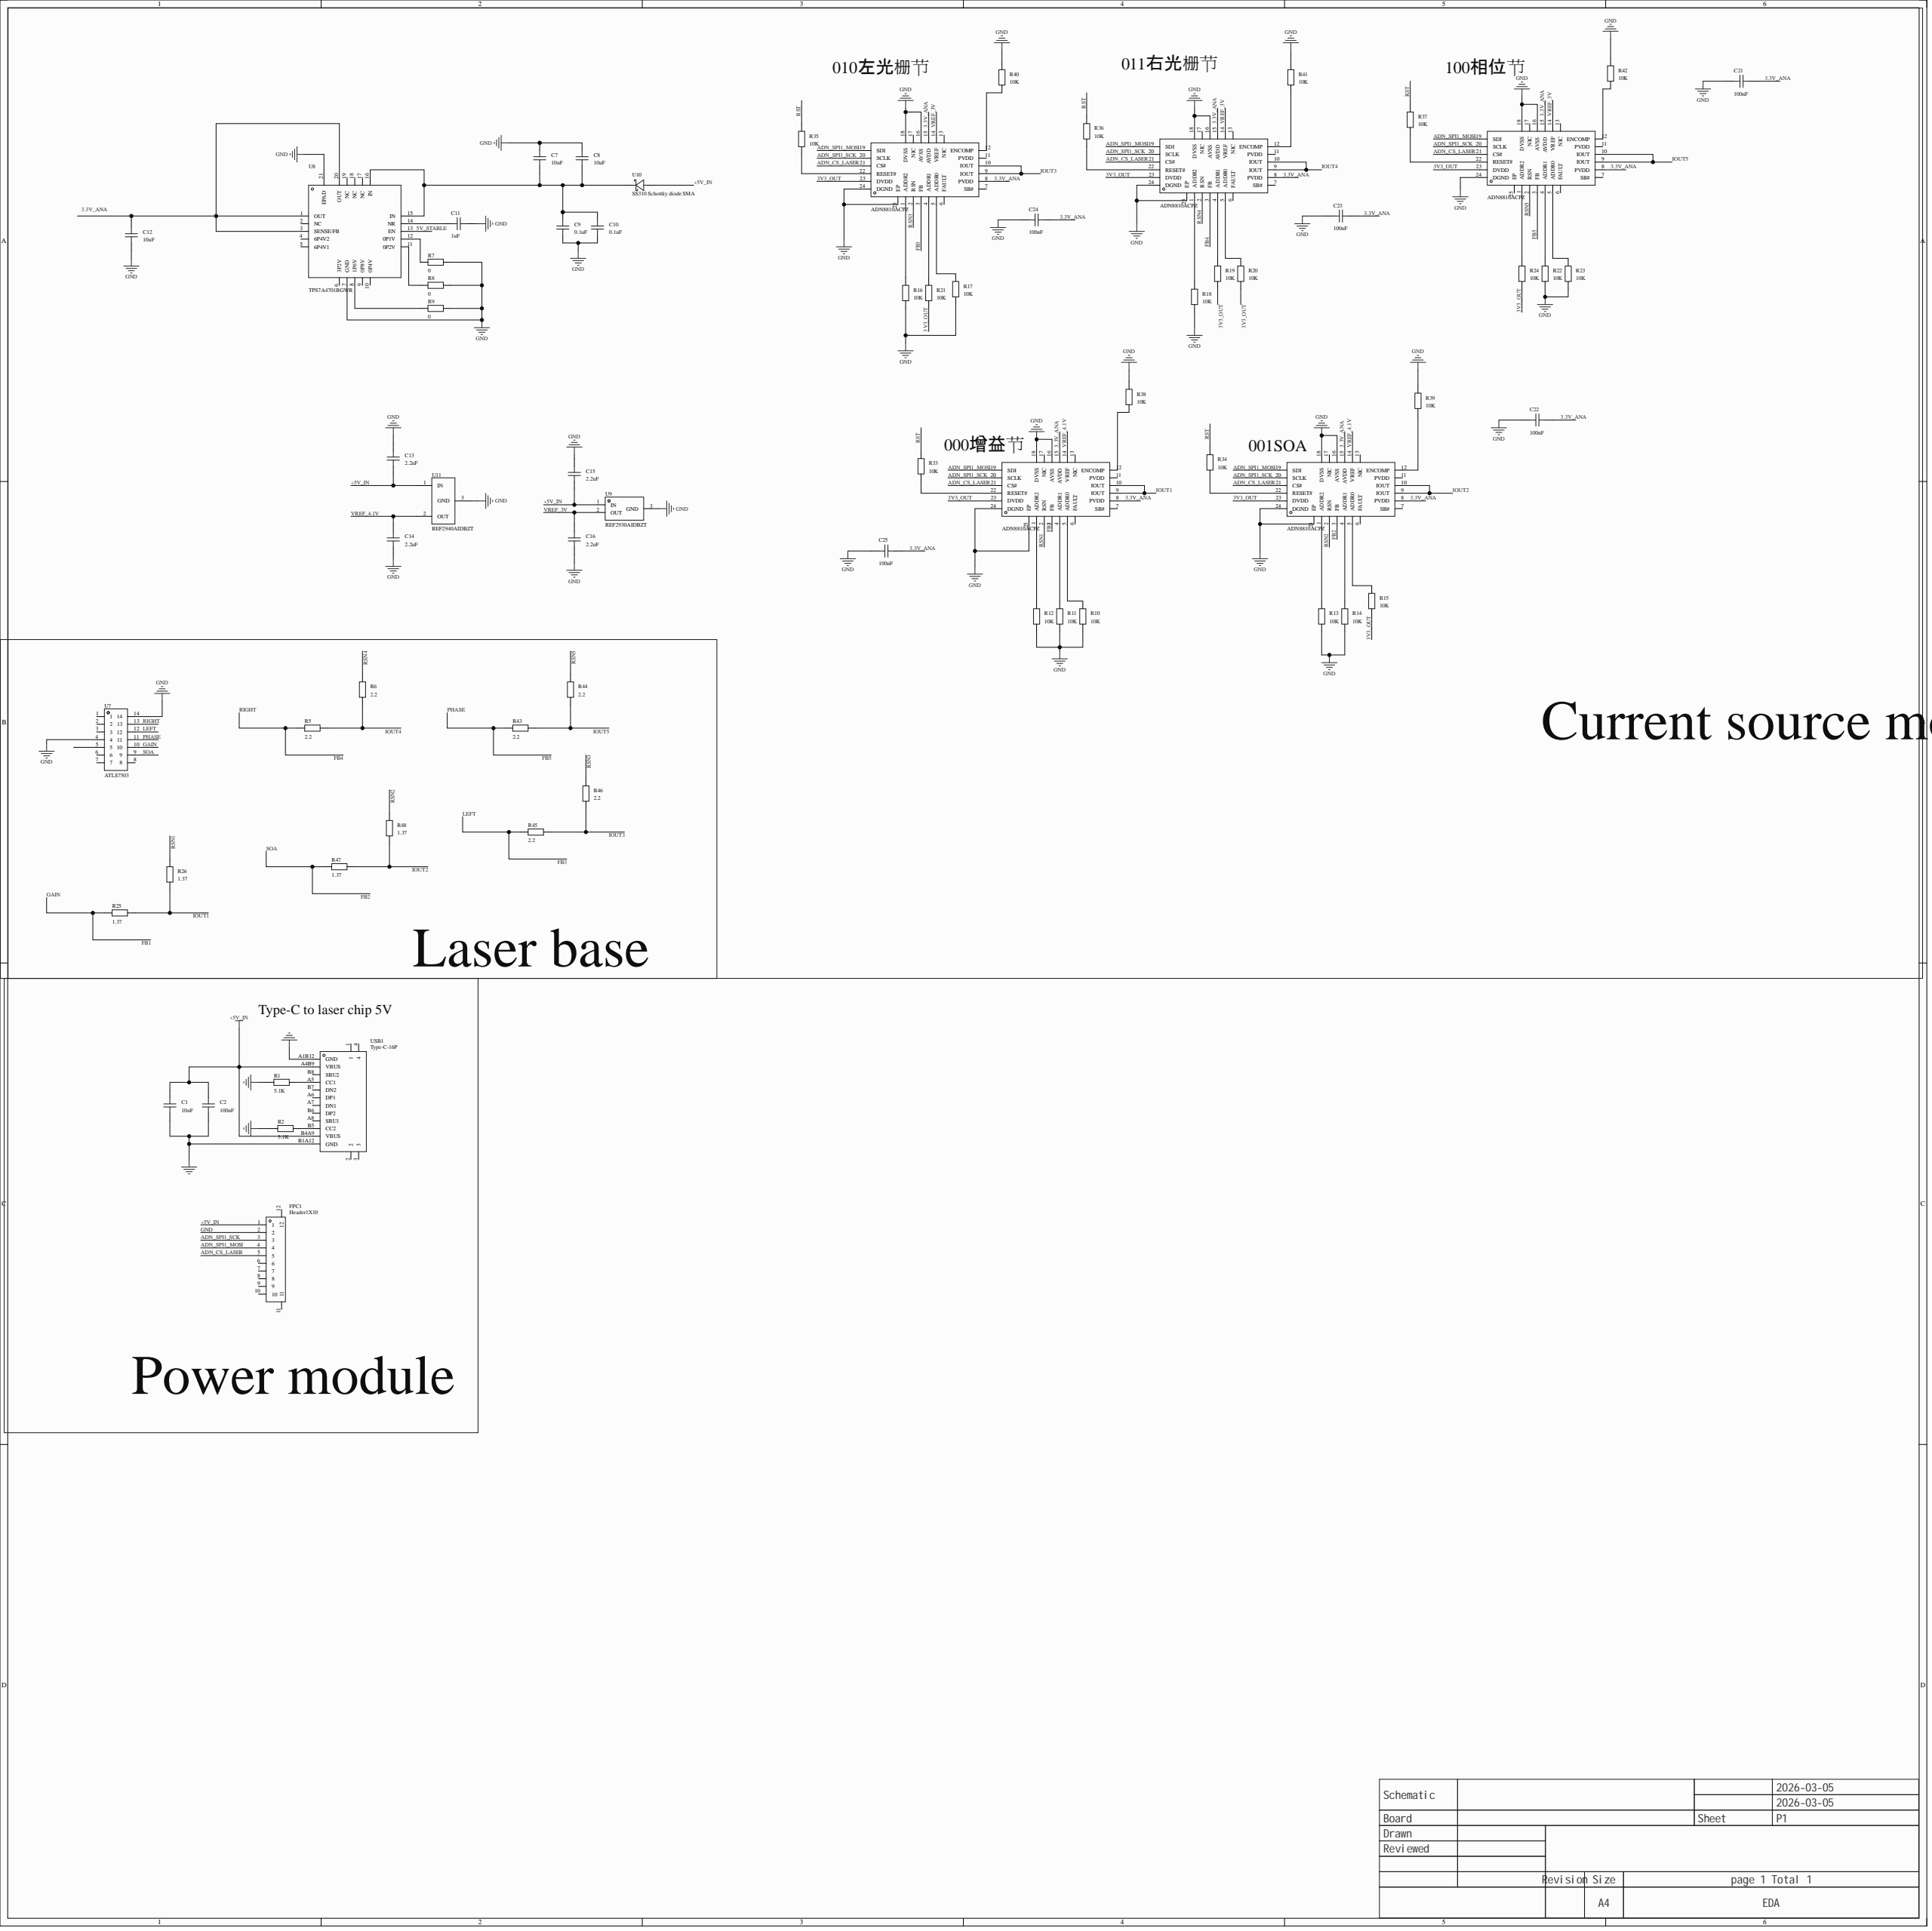Circuit board | Altium Designer | 69 parts | 58 nets
Bill of materials:
Comment,Description,Designator,Footprint,LibRef,Quantity
"ADN8810ACPZ","Output current: 300mA;","000增益节, 001SOA, 010左光栅节, 011右光栅节, 100相位节","LFCSP-24_L4.0-W4.0-P0.50-BL-EP2.3","ADN8810ACPZ","5"
"10uF","Capacitance: 10nF; accuracy: ±10%; rated voltage: 16V; temperature coefficient: X7R;","C1","C0402","AC0402KRX7R7BB103","1"
"100nF","Capacitance: 10nF; accuracy: ±10%; rated voltage: 16V; temperature coefficient: X7R;","C2","C0402","AC0402KRX7R7BB103","1"
"10uF","","C7, C8, C12","C0603","CAP_0603","3"
"0.1uF","","C9, C10","C0603","CAP_0603","2"
"1uF","","C11","C0603","CAP_0603","1"
"2.2uF","","C13, C14, C15, C16","C0603","CAP_0603","4"
"100nF","","C21, C22, C23, C24, C25","C0603","CAP_0603","5"
"Header1X10","","FPC1","FPC-SMD_10P-P1.00_C9900008955","Header1X10","1"
"5.1K","","R1, R2","R0603","Res_0603","2"
"2.2","","R5, R6, R43, R44, R45, R46","R0603","Res_0603","6"
"0","","R7, R8, R9","R0603","Res_0603","3"
"10K","","R10, R11, R12, R13, R14, R15, R16, R17, R18, R19, R20, R21, R22, R23, R24, R33, R34, R35, R36, R37, R38, R39, R40, R41, R42","R0603","Res_0603","25"
"1.37","","R25, R26, R47, R48","R0603","Res_0603","4"
"ATLS7503","","U7","HDR-SMD_14P-P1.27-V-F-R2-C7-LS4.8","HEADER7X2B","1"
"TPS7A4701RGWR","Output type: adjustable; working voltage: 35V; output voltage: 1.4V~34V; output current: 1A; power supply rejection ratio (PSRR): 78dB@(1kHz); output polarity: positive;","U8","VQFN-20_L5.0-W5.0-P0.65-TL-EP","TPS7A4701RGWR","1"
"REF2930AIDBZT","Output type: fixed; working voltage: 3.05V~5.5V; output voltage: 3V; output current: 25mA; accuracy: ±2%;","U9","SOT-23-3_L2.9-W1.3-P1.90-LS2.4-BR","REF2930AIDBZT","1"
"SS310 Schottky diode SMA","","U10","SMA_L4.3-W2.6-LS5.1-R-RD","SS310肖特基二极管SMA","1"
"REF2940AIDBZT","Output type: fixed; input voltage: 4.146V~5.5V; output voltage: 4.096V; output current: 25mA; accuracy: ±2%;","U11","SOT-23-3_L2.9-W1.3-P1.90-LS2.4-BR","REF2940AIDBZT","1"
"Type-C-16P","","USB1","USB-C-SMD_GT-USB-7010E","Type-C-16P","1"
Netlist (Protel format):
[
000增益节
LFCSP-24_L4.0-W4.0-P0.50-BL-EP2.3
ADN8810ACPZ



]
[
001SOA
LFCSP-24_L4.0-W4.0-P0.50-BL-EP2.3
ADN8810ACPZ



]
[
010左光栅节
LFCSP-24_L4.0-W4.0-P0.50-BL-EP2.3
ADN8810ACPZ



]
[
011右光栅节
LFCSP-24_L4.0-W4.0-P0.50-BL-EP2.3
ADN8810ACPZ



]
[
100相位节
LFCSP-24_L4.0-W4.0-P0.50-BL-EP2.3
ADN8810ACPZ



]
[
C1
C0402
10uF



]
[
C2
C0402
100nF



]
[
C7
C0603
10uF



]
[
C8
C0603
10uF



]
[
C9
C0603
0.1uF



]
[
C10
C0603
0.1uF



]
[
C11
C0603
1uF



]
[
C12
C0603
10uF



]
[
C13
C0603
2.2uF



]
[
C14
C0603
2.2uF



]
[
C15
C0603
2.2uF



]
[
C16
C0603
2.2uF



]
[
C21
C0603
100nF



]
[
C22
C0603
100nF



]
[
C23
C0603
100nF



]
[
C24
C0603
100nF



]
[
C25
C0603
100nF



]
[
FPC1
FPC-SMD_10P-P1.00_C9900008955
Header1X10



]
[
R1
R0603
5.1K



]
[
R2
R0603
5.1K



]
[
R5
R0603
2.2



]
[
R6
R0603
2.2



]
[
R7
R0603
0



]
[
R8
R0603
0



]
[
R9
R0603
0



]
[
R10
R0603
10K



]
[
R11
R0603
10K



]
[
R12
R0603
10K



]
[
R13
R0603
10K



]
[
R14
R0603
10K



]
[
R15
R0603
10K



]
[
R16
R0603
10K



]
[
R17
R0603
10K



]
[
R18
R0603
10K



]
[
R19
R0603
10K



]
[
R20
R0603
10K



]
[
R21
R0603
10K



]
[
R22
R0603
10K



]
[
R23
R0603
10K



]
[
R24
R0603
10K



]
[
R25
R0603
1.37



]
[
R26
R0603
1.37



]
[
R33
R0603
10K



]
[
R34
R0603
10K



]
[
R35
R0603
10K



]
[
R36
R0603
10K



]
[
R37
R0603
10K



]
[
R38
R0603
10K



]
[
R39
R0603
10K



]
[
R40
R0603
10K



]
[
R41
R0603
10K



]
[
R42
R0603
10K



]
[
R43
R0603
2.2



]
[
R44
R0603
2.2



]
[
R45
R0603
2.2



]
[
R46
R0603
2.2



]
[
R47
R0603
1.37



]
[
R48
R0603
1.37



]
[
U7
HDR-SMD_14P-P1.27-V-F-R2-C7-LS4.8
ATLS7503



]
[
U8
VQFN-20_L5.0-W5.0-P0.65-TL-EP
TPS7A4701RGWR



]
[
U9
SOT-23-3_L2.9-W1.3-P1.90-LS2.4-BR
REF2930AIDBZT



]
[
U10
SMA_L4.3-W2.6-LS5.1-R-RD
SS310 Schottky diode SMA



]
[
U11
SOT-23-3_L2.9-W1.3-P1.90-LS2.4-BR
REF2940AIDBZT



]
[
USB1
USB-C-SMD_GT-USB-7010E
Type-C-16P



]
(
VREF_4.1V
000增益节-14
001SOA-14
C14-2
U11-2
)
(
VREF_3V
010左光栅节-14
011右光栅节-14
100相位节-14
C16-2
U9-2
)
(
RST
R33-2
R34-2
R35-2
R36-2
R37-2
)
(
RSN5
100相位节-2
R44-1
)
(
RSN4
011右光栅节-2
R6-1
)
(
RSN3
010左光栅节-2
R46-1
)
(
RSN2
001SOA-2
R48-1
)
(
RSN1
000增益节-2
R26-1
)
(
NetR9_1
R9-1
U8-8
)
(
NetR8_1
R8-1
U8-11
)
(
NetR7_1
R7-1
U8-12
)
(
NetR2_2
R2-2
USB1-B5
)
(
NetR1_2
R1-2
USB1-A5
)
(
NetC12_2
C12-2
U8-1
U8-3
U8-20
)
(
NetC11_2
C11-2
U8-14
)
(
NetC7_1
C7-1
C8-1
C9-2
C10-2
U8-15
U8-16
U10-2
)
(
Net100相位节_22
100相位节-22
R37-1
)
(
Net100相位节_12
100相位节-12
R42-1
)
(
Net100相位节_5
100相位节-5
R23-2
)
(
Net100相位节_4
100相位节-4
R22-2
)
(
Net100相位节_1
100相位节-1
R24-2
)
(
Net011右光栅节_22
011右光栅节-22
R36-1
)
(
Net011右光栅节_12
011右光栅节-12
R41-1
)
(
Net011右光栅节_5
011右光栅节-5
R20-2
)
(
Net011右光栅节_4
011右光栅节-4
R19-2
)
(
Net011右光栅节_1
011右光栅节-1
R18-2
)
(
Net010左光栅节_22
010左光栅节-22
R35-1
)
(
Net010左光栅节_12
010左光栅节-12
R40-1
)
(
Net010左光栅节_5
010左光栅节-5
R17-2
)
(
Net010左光栅节_4
010左光栅节-4
R21-2
)
(
Net010左光栅节_1
010左光栅节-1
R16-2
)
(
Net001SOA_22
001SOA-22
R34-1
)
(
Net001SOA_12
001SOA-12
R39-1
)
(
Net001SOA_5
001SOA-5
R15-2
)
(
Net001SOA_4
001SOA-4
R14-2
)
(
Net001SOA_1
001SOA-1
R13-2
)
(
Net000增益节_22
000增益节-22
R33-1
)
(
Net000增益节_12
000增益节-12
R38-1
)
(
Net000增益节_5
000增益节-5
R10-2
)
(
Net000增益节_4
000增益节-4
R11-2
)
(
Net000增益节_1
000增益节-1
R12-2
)
(
IOUT5
100相位节-9
100相位节-10
R43-1
R44-2
)
(
IOUT4
011右光栅节-9
011右光栅节-10
R5-1
R6-2
)
(
IOUT3
010左光栅节-9
010左光栅节-10
R45-1
R46-2
)
(
IOUT2
001SOA-9
001SOA-10
R47-1
R48-2
)
(
IOUT1
000增益节-9
000增益节-10
R25-1
R26-2
)
(
GND
000增益节-16
000增益节-18
000增益节-24
000增益节-25
001SOA-16
001SOA-18
001SOA-24
001SOA-25
010左光栅节-16
010左光栅节-18
010左光栅节-24
010左光栅节-25
011右光栅节-16
011右光栅节-18
011右光栅节-24
011右光栅节-25
100相位节-16
100相位节-18
100相位节-24
C1-1
C2-1
C7-2
C8-2
C9-1
C10-1
C11-1
C12-1
C13-2
C14-1
C15-2
C16-1
C21-2
C22-2
C23-2
C24-2
C25-2
FPC1-2
R1-1
R2-1
R7-2
R8-2
R9-2
R10-1
R11-1
R12-1
R13-1
R14-1
R16-1
R17-1
R18-1
R22-1
R23-1
R38-2
R39-2
R40-2
R41-2
R42-2
U7-4
U7-14
U8-7
U8-21
U9-3
U11-3
USB1-A1B12
USB1-B1A12
)
(
FB5
100相位节-3
R43-2
U7-11
)
(
FB4
011右光栅节-3
R5-2
U7-13
)
(
FB3
010左光栅节-3
R45-2
U7-12
)
(
FB2
001SOA-3
R47-2
U7-9
)
(
FB1
000增益节-3
R25-2
U7-10
)
(
ADN_SPI1_SCK
000增益节-20
001SOA-20
010左光栅节-20
011右光栅节-20
100相位节-20
FPC1-3
)
(
ADN_SPI1_MOSI
000增益节-19
001SOA-19
010左光栅节-19
011右光栅节-19
100相位节-19
FPC1-4
)
(
ADN_CS_LASER
000增益节-21
001SOA-21
010左光栅节-21
011右光栅节-21
100相位节-21
FPC1-5
)
(
+5V_IN
C1-2
C2-2
C13-1
C15-1
FPC1-1
U9-1
U10-1
U11-1
USB1-A4B9
USB1-B4A9
)
(
3V3_OUT
000增益节-23
001SOA-23
010左光栅节-23
011右光栅节-23
100相位节-23
R15-1
R19-1
R20-1
R21-1
R24-1
)
(
3.3V_ANA
000增益节-8
000增益节-15
001SOA-8
001SOA-15
010左光栅节-8
010左光栅节-15
011右光栅节-8
011右光栅节-15
100相位节-8
100相位节-15
C21-1
C22-1
C23-1
C24-1
C25-1
)